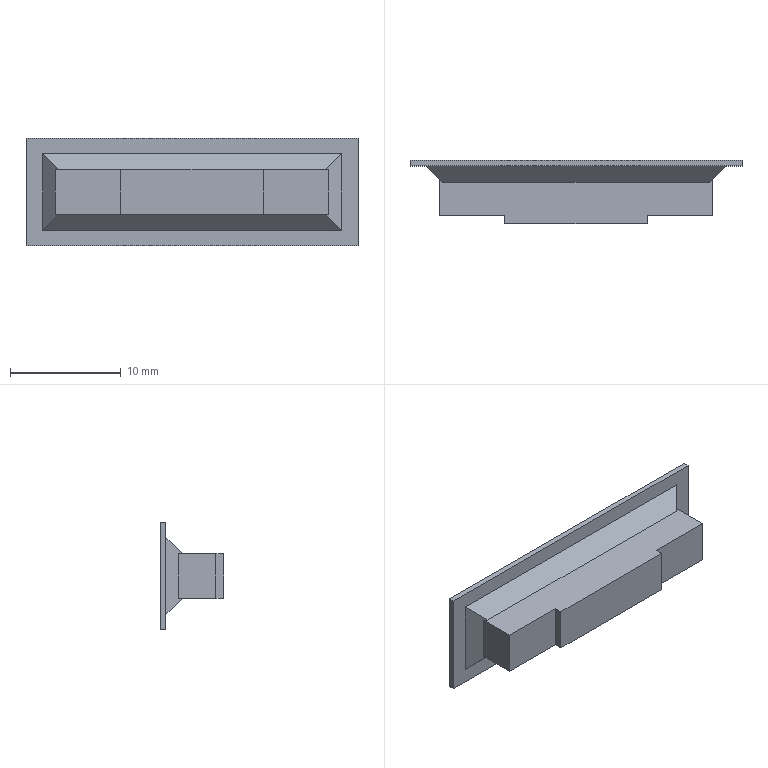Part | NX | 1 solid | 24 faces | box 30 x 5.7 x 9.7 mm | volume 631.13 mm3 | plane 24
STEP:
#1=CARTESIAN_POINT('',(12.05,-1.95,2.));
#2=VERTEX_POINT('',#1);
#3=CARTESIAN_POINT('',(-12.05,-1.95,2.));
#4=VERTEX_POINT('',#3);
#5=CARTESIAN_POINT('',(13.5,-1.95,2.));
#6=DIRECTION('',(-1.,0.,0.));
#7=VECTOR('',#6,1000.);
#8=LINE('',#5,#7);
#9=EDGE_CURVE('',#2,#4,#8,.T.);
#10=ORIENTED_EDGE('',*,*,#9,.F.);
#11=CARTESIAN_POINT('',(13.5,-0.5,3.45));
#12=VERTEX_POINT('',#11);
#13=CARTESIAN_POINT('',(13.5,-0.5,3.45));
#14=DIRECTION('',(0.5774,0.5774,0.5774));
#15=VECTOR('',#14,1000.);
#16=LINE('',#13,#15);
#17=EDGE_CURVE('',#2,#12,#16,.T.);
#18=ORIENTED_EDGE('',*,*,#17,.T.);
#19=CARTESIAN_POINT('',(-13.5,-0.5,3.45));
#20=VERTEX_POINT('',#19);
#21=CARTESIAN_POINT('',(13.5,-0.5,3.45));
#22=DIRECTION('',(-1.,0.,0.));
#23=VECTOR('',#22,1000.);
#24=LINE('',#21,#23);
#25=EDGE_CURVE('',#12,#20,#24,.T.);
#26=ORIENTED_EDGE('',*,*,#25,.T.);
#27=CARTESIAN_POINT('',(-4.5,-9.5,-5.55));
#28=DIRECTION('',(0.5774,-0.5774,-0.5774));
#29=VECTOR('',#28,1000.);
#30=LINE('',#27,#29);
#31=EDGE_CURVE('',#20,#4,#30,.T.);
#32=ORIENTED_EDGE('',*,*,#31,.T.);
#33=EDGE_LOOP('',(#10,#18,#26,#32));
#34=FACE_BOUND('',#33,.T.);
#35=CARTESIAN_POINT('',(13.5,-0.5,3.45));
#36=DIRECTION('',(0.,0.7071,-0.7071));
#37=DIRECTION('',(0.,0.7071,0.7071));
#38=AXIS2_PLACEMENT_3D('',#35,#36,#37);
#39=PLANE('',#38);
#40=ADVANCED_FACE('',(#34),#39,.F.);
#41=CARTESIAN_POINT('',(-12.05,-1.95,-2.));
#42=VERTEX_POINT('',#41);
#43=CARTESIAN_POINT('',(12.05,-1.95,-2.));
#44=VERTEX_POINT('',#43);
#45=CARTESIAN_POINT('',(13.5,-1.95,-2.));
#46=DIRECTION('',(1.,0.,0.));
#47=VECTOR('',#46,1000.);
#48=LINE('',#45,#47);
#49=EDGE_CURVE('',#42,#44,#48,.T.);
#50=ORIENTED_EDGE('',*,*,#49,.F.);
#51=CARTESIAN_POINT('',(-13.5,-0.5,-3.45));
#52=VERTEX_POINT('',#51);
#53=CARTESIAN_POINT('',(-4.5,-9.5,5.55));
#54=DIRECTION('',(-0.5774,0.5774,-0.5774));
#55=VECTOR('',#54,1000.);
#56=LINE('',#53,#55);
#57=EDGE_CURVE('',#42,#52,#56,.T.);
#58=ORIENTED_EDGE('',*,*,#57,.T.);
#59=CARTESIAN_POINT('',(13.5,-0.5,-3.45));
#60=VERTEX_POINT('',#59);
#61=CARTESIAN_POINT('',(13.5,-0.5,-3.45));
#62=DIRECTION('',(-1.,0.,0.));
#63=VECTOR('',#62,1000.);
#64=LINE('',#61,#63);
#65=EDGE_CURVE('',#60,#52,#64,.T.);
#66=ORIENTED_EDGE('',*,*,#65,.F.);
#67=CARTESIAN_POINT('',(13.5,-0.5,-3.45));
#68=DIRECTION('',(-0.5774,-0.5774,0.5774));
#69=VECTOR('',#68,1000.);
#70=LINE('',#67,#69);
#71=EDGE_CURVE('',#60,#44,#70,.T.);
#72=ORIENTED_EDGE('',*,*,#71,.T.);
#73=EDGE_LOOP('',(#50,#58,#66,#72));
#74=FACE_BOUND('',#73,.T.);
#75=CARTESIAN_POINT('',(13.5,-0.5,-3.45));
#76=DIRECTION('',(0.,0.7071,0.7071));
#77=DIRECTION('',(0.,-0.7071,0.7071));
#78=AXIS2_PLACEMENT_3D('',#75,#76,#77);
#79=PLANE('',#78);
#80=ADVANCED_FACE('',(#74),#79,.F.);
#81=CARTESIAN_POINT('',(12.35,-1.65,2.));
#82=VERTEX_POINT('',#81);
#83=CARTESIAN_POINT('',(13.5,-0.5,2.));
#84=DIRECTION('',(-0.7071,-0.7071,0.));
#85=VECTOR('',#84,1000.);
#86=LINE('',#83,#85);
#87=EDGE_CURVE('',#82,#2,#86,.T.);
#88=ORIENTED_EDGE('',*,*,#87,.F.);
#89=CARTESIAN_POINT('',(12.35,-1.65,-2.));
#90=VERTEX_POINT('',#89);
#91=CARTESIAN_POINT('',(12.35,-1.65,-4.85));
#92=DIRECTION('',(0.,0.,1.));
#93=VECTOR('',#92,1000.);
#94=LINE('',#91,#93);
#95=EDGE_CURVE('',#90,#82,#94,.T.);
#96=ORIENTED_EDGE('',*,*,#95,.F.);
#97=CARTESIAN_POINT('',(13.5,-0.5,-2.));
#98=DIRECTION('',(0.7071,0.7071,0.));
#99=VECTOR('',#98,1000.);
#100=LINE('',#97,#99);
#101=EDGE_CURVE('',#44,#90,#100,.T.);
#102=ORIENTED_EDGE('',*,*,#101,.F.);
#103=ORIENTED_EDGE('',*,*,#71,.F.);
#104=CARTESIAN_POINT('',(13.5,-0.5,3.45));
#105=DIRECTION('',(0.,0.,1.));
#106=VECTOR('',#105,1000.);
#107=LINE('',#104,#106);
#108=EDGE_CURVE('',#60,#12,#107,.T.);
#109=ORIENTED_EDGE('',*,*,#108,.T.);
#110=ORIENTED_EDGE('',*,*,#17,.F.);
#111=EDGE_LOOP('',(#88,#96,#102,#103,#109,#110));
#112=FACE_BOUND('',#111,.T.);
#113=CARTESIAN_POINT('',(13.5,-0.5,-4.85));
#114=DIRECTION('',(-0.7071,0.7071,0.));
#115=DIRECTION('',(-0.7071,-0.7071,0.));
#116=AXIS2_PLACEMENT_3D('',#113,#114,#115);
#117=PLANE('',#116);
#118=ADVANCED_FACE('',(#112),#117,.F.);
#119=CARTESIAN_POINT('',(-12.35,-1.65,2.));
#120=VERTEX_POINT('',#119);
#121=CARTESIAN_POINT('',(-13.5,-0.5,2.));
#122=DIRECTION('',(-0.7071,0.7071,0.));
#123=VECTOR('',#122,1000.);
#124=LINE('',#121,#123);
#125=EDGE_CURVE('',#4,#120,#124,.T.);
#126=ORIENTED_EDGE('',*,*,#125,.F.);
#127=ORIENTED_EDGE('',*,*,#31,.F.);
#128=CARTESIAN_POINT('',(-13.5,-0.5,3.45));
#129=DIRECTION('',(0.,0.,1.));
#130=VECTOR('',#129,1000.);
#131=LINE('',#128,#130);
#132=EDGE_CURVE('',#52,#20,#131,.T.);
#133=ORIENTED_EDGE('',*,*,#132,.F.);
#134=ORIENTED_EDGE('',*,*,#57,.F.);
#135=CARTESIAN_POINT('',(-12.35,-1.65,-2.));
#136=VERTEX_POINT('',#135);
#137=CARTESIAN_POINT('',(-13.5,-0.5,-2.));
#138=DIRECTION('',(0.7071,-0.7071,0.));
#139=VECTOR('',#138,1000.);
#140=LINE('',#137,#139);
#141=EDGE_CURVE('',#136,#42,#140,.T.);
#142=ORIENTED_EDGE('',*,*,#141,.F.);
#143=CARTESIAN_POINT('',(-12.35,-1.65,-4.85));
#144=DIRECTION('',(0.,0.,-1.));
#145=VECTOR('',#144,1000.);
#146=LINE('',#143,#145);
#147=EDGE_CURVE('',#120,#136,#146,.T.);
#148=ORIENTED_EDGE('',*,*,#147,.F.);
#149=EDGE_LOOP('',(#126,#127,#133,#134,#142,#148));
#150=FACE_BOUND('',#149,.T.);
#151=CARTESIAN_POINT('',(-13.5,-0.5,-4.85));
#152=DIRECTION('',(0.7071,0.7071,0.));
#153=DIRECTION('',(-0.7071,0.7071,0.));
#154=AXIS2_PLACEMENT_3D('',#151,#152,#153);
#155=PLANE('',#154);
#156=ADVANCED_FACE('',(#150),#155,.F.);
#157=ORIENTED_EDGE('',*,*,#132,.T.);
#158=ORIENTED_EDGE('',*,*,#25,.F.);
#159=ORIENTED_EDGE('',*,*,#108,.F.);
#160=ORIENTED_EDGE('',*,*,#65,.T.);
#161=EDGE_LOOP('',(#157,#158,#159,#160));
#162=FACE_BOUND('',#161,.T.);
#163=CARTESIAN_POINT('',(15.,-0.5,4.85));
#164=VERTEX_POINT('',#163);
#165=CARTESIAN_POINT('',(15.,-0.5,-4.85));
#166=VERTEX_POINT('',#165);
#167=CARTESIAN_POINT('',(15.,-0.5,-4.85));
#168=DIRECTION('',(0.,0.,-1.));
#169=VECTOR('',#168,1000.);
#170=LINE('',#167,#169);
#171=EDGE_CURVE('',#164,#166,#170,.T.);
#172=ORIENTED_EDGE('',*,*,#171,.F.);
#173=CARTESIAN_POINT('',(-15.,-0.5,4.85));
#174=VERTEX_POINT('',#173);
#175=CARTESIAN_POINT('',(-15.,-0.5,4.85));
#176=DIRECTION('',(1.,0.,0.));
#177=VECTOR('',#176,1000.);
#178=LINE('',#175,#177);
#179=EDGE_CURVE('',#174,#164,#178,.T.);
#180=ORIENTED_EDGE('',*,*,#179,.F.);
#181=CARTESIAN_POINT('',(-15.,-0.5,-4.85));
#182=VERTEX_POINT('',#181);
#183=CARTESIAN_POINT('',(-15.,-0.5,-4.85));
#184=DIRECTION('',(0.,0.,1.));
#185=VECTOR('',#184,1000.);
#186=LINE('',#183,#185);
#187=EDGE_CURVE('',#182,#174,#186,.T.);
#188=ORIENTED_EDGE('',*,*,#187,.F.);
#189=CARTESIAN_POINT('',(-15.,-0.5,-4.85));
#190=DIRECTION('',(-1.,0.,0.));
#191=VECTOR('',#190,1000.);
#192=LINE('',#189,#191);
#193=EDGE_CURVE('',#166,#182,#192,.T.);
#194=ORIENTED_EDGE('',*,*,#193,.F.);
#195=EDGE_LOOP('',(#172,#180,#188,#194));
#196=FACE_BOUND('',#195,.T.);
#197=CARTESIAN_POINT('',(-15.,-0.5,4.85));
#198=DIRECTION('',(0.,1.,0.));
#199=DIRECTION('',(0.,0.,1.));
#200=AXIS2_PLACEMENT_3D('',#197,#198,#199);
#201=PLANE('',#200);
#202=ADVANCED_FACE('',(#162,#196),#201,.F.);
#203=CARTESIAN_POINT('',(-15.,0.,-4.85));
#204=VERTEX_POINT('',#203);
#205=CARTESIAN_POINT('',(-15.,0.,4.85));
#206=VERTEX_POINT('',#205);
#207=CARTESIAN_POINT('',(-15.,0.,-4.85));
#208=DIRECTION('',(0.,0.,1.));
#209=VECTOR('',#208,1000.);
#210=LINE('',#207,#209);
#211=EDGE_CURVE('',#204,#206,#210,.T.);
#212=ORIENTED_EDGE('',*,*,#211,.F.);
#213=CARTESIAN_POINT('',(-15.,-0.5,-4.85));
#214=DIRECTION('',(0.,1.,0.));
#215=VECTOR('',#214,1000.);
#216=LINE('',#213,#215);
#217=EDGE_CURVE('',#182,#204,#216,.T.);
#218=ORIENTED_EDGE('',*,*,#217,.F.);
#219=ORIENTED_EDGE('',*,*,#187,.T.);
#220=CARTESIAN_POINT('',(-15.,-0.5,4.85));
#221=DIRECTION('',(0.,1.,0.));
#222=VECTOR('',#221,1000.);
#223=LINE('',#220,#222);
#224=EDGE_CURVE('',#174,#206,#223,.T.);
#225=ORIENTED_EDGE('',*,*,#224,.T.);
#226=EDGE_LOOP('',(#212,#218,#219,#225));
#227=FACE_BOUND('',#226,.T.);
#228=CARTESIAN_POINT('',(-15.,-0.5,-4.85));
#229=DIRECTION('',(-1.,0.,0.));
#230=DIRECTION('',(0.,0.,1.));
#231=AXIS2_PLACEMENT_3D('',#228,#229,#230);
#232=PLANE('',#231);
#233=ADVANCED_FACE('',(#227),#232,.T.);
#234=CARTESIAN_POINT('',(15.,0.,-4.85));
#235=VERTEX_POINT('',#234);
#236=CARTESIAN_POINT('',(-15.,0.,-4.85));
#237=DIRECTION('',(-1.,0.,0.));
#238=VECTOR('',#237,1000.);
#239=LINE('',#236,#238);
#240=EDGE_CURVE('',#235,#204,#239,.T.);
#241=ORIENTED_EDGE('',*,*,#240,.F.);
#242=CARTESIAN_POINT('',(15.,-0.5,-4.85));
#243=DIRECTION('',(0.,1.,0.));
#244=VECTOR('',#243,1000.);
#245=LINE('',#242,#244);
#246=EDGE_CURVE('',#166,#235,#245,.T.);
#247=ORIENTED_EDGE('',*,*,#246,.F.);
#248=ORIENTED_EDGE('',*,*,#193,.T.);
#249=ORIENTED_EDGE('',*,*,#217,.T.);
#250=EDGE_LOOP('',(#241,#247,#248,#249));
#251=FACE_BOUND('',#250,.T.);
#252=CARTESIAN_POINT('',(-15.,-0.5,-4.85));
#253=DIRECTION('',(0.,0.,-1.));
#254=DIRECTION('',(-1.,0.,0.));
#255=AXIS2_PLACEMENT_3D('',#252,#253,#254);
#256=PLANE('',#255);
#257=ADVANCED_FACE('',(#251),#256,.T.);
#258=CARTESIAN_POINT('',(15.,0.,4.85));
#259=VERTEX_POINT('',#258);
#260=CARTESIAN_POINT('',(15.,0.,-4.85));
#261=DIRECTION('',(0.,0.,-1.));
#262=VECTOR('',#261,1000.);
#263=LINE('',#260,#262);
#264=EDGE_CURVE('',#259,#235,#263,.T.);
#265=ORIENTED_EDGE('',*,*,#264,.F.);
#266=CARTESIAN_POINT('',(15.,-0.5,4.85));
#267=DIRECTION('',(0.,1.,0.));
#268=VECTOR('',#267,1000.);
#269=LINE('',#266,#268);
#270=EDGE_CURVE('',#164,#259,#269,.T.);
#271=ORIENTED_EDGE('',*,*,#270,.F.);
#272=ORIENTED_EDGE('',*,*,#171,.T.);
#273=ORIENTED_EDGE('',*,*,#246,.T.);
#274=EDGE_LOOP('',(#265,#271,#272,#273));
#275=FACE_BOUND('',#274,.T.);
#276=CARTESIAN_POINT('',(15.,-0.5,-4.85));
#277=DIRECTION('',(1.,0.,0.));
#278=DIRECTION('',(0.,0.,-1.));
#279=AXIS2_PLACEMENT_3D('',#276,#277,#278);
#280=PLANE('',#279);
#281=ADVANCED_FACE('',(#275),#280,.T.);
#282=CARTESIAN_POINT('',(-15.,0.,4.85));
#283=DIRECTION('',(1.,0.,0.));
#284=VECTOR('',#283,1000.);
#285=LINE('',#282,#284);
#286=EDGE_CURVE('',#206,#259,#285,.T.);
#287=ORIENTED_EDGE('',*,*,#286,.F.);
#288=ORIENTED_EDGE('',*,*,#224,.F.);
#289=ORIENTED_EDGE('',*,*,#179,.T.);
#290=ORIENTED_EDGE('',*,*,#270,.T.);
#291=EDGE_LOOP('',(#287,#288,#289,#290));
#292=FACE_BOUND('',#291,.T.);
#293=CARTESIAN_POINT('',(-15.,-0.5,4.85));
#294=DIRECTION('',(0.,0.,1.));
#295=DIRECTION('',(1.,0.,0.));
#296=AXIS2_PLACEMENT_3D('',#293,#294,#295);
#297=PLANE('',#296);
#298=ADVANCED_FACE('',(#292),#297,.T.);
#299=CARTESIAN_POINT('',(10.5,0.,2.1));
#300=VERTEX_POINT('',#299);
#301=CARTESIAN_POINT('',(10.5,0.,-2.1));
#302=VERTEX_POINT('',#301);
#303=CARTESIAN_POINT('',(10.5,0.,-2.1));
#304=DIRECTION('',(0.,0.,-1.));
#305=VECTOR('',#304,1000.);
#306=LINE('',#303,#305);
#307=EDGE_CURVE('',#300,#302,#306,.T.);
#308=ORIENTED_EDGE('',*,*,#307,.F.);
#309=CARTESIAN_POINT('',(-10.5,0.,2.1));
#310=VERTEX_POINT('',#309);
#311=CARTESIAN_POINT('',(10.5,0.,2.1));
#312=DIRECTION('',(1.,0.,0.));
#313=VECTOR('',#312,1000.);
#314=LINE('',#311,#313);
#315=EDGE_CURVE('',#310,#300,#314,.T.);
#316=ORIENTED_EDGE('',*,*,#315,.F.);
#317=CARTESIAN_POINT('',(-10.5,0.,-2.1));
#318=VERTEX_POINT('',#317);
#319=CARTESIAN_POINT('',(-10.5,0.,-2.1));
#320=DIRECTION('',(0.,0.,1.));
#321=VECTOR('',#320,1000.);
#322=LINE('',#319,#321);
#323=EDGE_CURVE('',#318,#310,#322,.T.);
#324=ORIENTED_EDGE('',*,*,#323,.F.);
#325=CARTESIAN_POINT('',(10.5,0.,-2.1));
#326=DIRECTION('',(-1.,0.,0.));
#327=VECTOR('',#326,1000.);
#328=LINE('',#325,#327);
#329=EDGE_CURVE('',#302,#318,#328,.T.);
#330=ORIENTED_EDGE('',*,*,#329,.F.);
#331=EDGE_LOOP('',(#308,#316,#324,#330));
#332=FACE_BOUND('',#331,.T.);
#333=ORIENTED_EDGE('',*,*,#211,.T.);
#334=ORIENTED_EDGE('',*,*,#286,.T.);
#335=ORIENTED_EDGE('',*,*,#264,.T.);
#336=ORIENTED_EDGE('',*,*,#240,.T.);
#337=EDGE_LOOP('',(#333,#334,#335,#336));
#338=FACE_BOUND('',#337,.T.);
#339=CARTESIAN_POINT('',(-15.,0.,4.85));
#340=DIRECTION('',(0.,1.,0.));
#341=DIRECTION('',(0.,0.,1.));
#342=AXIS2_PLACEMENT_3D('',#339,#340,#341);
#343=PLANE('',#342);
#344=ADVANCED_FACE('',(#332,#338),#343,.T.);
#345=CARTESIAN_POINT('',(12.35,-5.,2.));
#346=VERTEX_POINT('',#345);
#347=CARTESIAN_POINT('',(12.35,-5.7,2.));
#348=DIRECTION('',(0.,1.,0.));
#349=VECTOR('',#348,1000.);
#350=LINE('',#347,#349);
#351=EDGE_CURVE('',#346,#82,#350,.T.);
#352=ORIENTED_EDGE('',*,*,#351,.F.);
#353=CARTESIAN_POINT('',(12.35,-5.,-2.));
#354=VERTEX_POINT('',#353);
#355=CARTESIAN_POINT('',(12.35,-5.,-7.941));
#356=DIRECTION('',(0.,0.,1.));
#357=VECTOR('',#356,1000.);
#358=LINE('',#355,#357);
#359=EDGE_CURVE('',#354,#346,#358,.T.);
#360=ORIENTED_EDGE('',*,*,#359,.F.);
#361=CARTESIAN_POINT('',(12.35,-5.7,-2.));
#362=DIRECTION('',(0.,1.,0.));
#363=VECTOR('',#362,1000.);
#364=LINE('',#361,#363);
#365=EDGE_CURVE('',#354,#90,#364,.T.);
#366=ORIENTED_EDGE('',*,*,#365,.T.);
#367=ORIENTED_EDGE('',*,*,#95,.T.);
#368=EDGE_LOOP('',(#352,#360,#366,#367));
#369=FACE_BOUND('',#368,.T.);
#370=CARTESIAN_POINT('',(12.35,-5.7,2.));
#371=DIRECTION('',(-1.,0.,0.));
#372=DIRECTION('',(0.,0.,1.));
#373=AXIS2_PLACEMENT_3D('',#370,#371,#372);
#374=PLANE('',#373);
#375=ADVANCED_FACE('',(#369),#374,.F.);
#376=CARTESIAN_POINT('',(6.45,-5.,2.));
#377=VERTEX_POINT('',#376);
#378=CARTESIAN_POINT('',(6.45,-5.7,2.));
#379=VERTEX_POINT('',#378);
#380=CARTESIAN_POINT('',(6.45,-5.,2.));
#381=DIRECTION('',(0.,-1.,0.));
#382=VECTOR('',#381,1000.);
#383=LINE('',#380,#382);
#384=EDGE_CURVE('',#377,#379,#383,.T.);
#385=ORIENTED_EDGE('',*,*,#384,.F.);
#386=CARTESIAN_POINT('',(12.35,-5.,2.));
#387=DIRECTION('',(-1.,0.,0.));
#388=VECTOR('',#387,1000.);
#389=LINE('',#386,#388);
#390=EDGE_CURVE('',#346,#377,#389,.T.);
#391=ORIENTED_EDGE('',*,*,#390,.F.);
#392=ORIENTED_EDGE('',*,*,#351,.T.);
#393=ORIENTED_EDGE('',*,*,#87,.T.);
#394=ORIENTED_EDGE('',*,*,#9,.T.);
#395=ORIENTED_EDGE('',*,*,#125,.T.);
#396=CARTESIAN_POINT('',(-12.35,-5.,2.));
#397=VERTEX_POINT('',#396);
#398=CARTESIAN_POINT('',(-12.35,-5.7,2.));
#399=DIRECTION('',(0.,1.,0.));
#400=VECTOR('',#399,1000.);
#401=LINE('',#398,#400);
#402=EDGE_CURVE('',#397,#120,#401,.T.);
#403=ORIENTED_EDGE('',*,*,#402,.F.);
#404=CARTESIAN_POINT('',(-6.45,-5.,2.));
#405=VERTEX_POINT('',#404);
#406=CARTESIAN_POINT('',(-12.35,-5.,2.));
#407=DIRECTION('',(-1.,0.,0.));
#408=VECTOR('',#407,1000.);
#409=LINE('',#406,#408);
#410=EDGE_CURVE('',#405,#397,#409,.T.);
#411=ORIENTED_EDGE('',*,*,#410,.F.);
#412=CARTESIAN_POINT('',(-6.45,-5.7,2.));
#413=VERTEX_POINT('',#412);
#414=CARTESIAN_POINT('',(-6.45,-5.,2.));
#415=DIRECTION('',(0.,1.,0.));
#416=VECTOR('',#415,1000.);
#417=LINE('',#414,#416);
#418=EDGE_CURVE('',#413,#405,#417,.T.);
#419=ORIENTED_EDGE('',*,*,#418,.F.);
#420=CARTESIAN_POINT('',(12.35,-5.7,2.));
#421=DIRECTION('',(-1.,0.,0.));
#422=VECTOR('',#421,1000.);
#423=LINE('',#420,#422);
#424=EDGE_CURVE('',#379,#413,#423,.T.);
#425=ORIENTED_EDGE('',*,*,#424,.F.);
#426=EDGE_LOOP('',(#385,#391,#392,#393,#394,#395,#403,#411,#419,#425));
#427=FACE_BOUND('',#426,.T.);
#428=CARTESIAN_POINT('',(12.35,-5.7,2.));
#429=DIRECTION('',(0.,0.,-1.));
#430=DIRECTION('',(-1.,0.,0.));
#431=AXIS2_PLACEMENT_3D('',#428,#429,#430);
#432=PLANE('',#431);
#433=ADVANCED_FACE('',(#427),#432,.F.);
#434=CARTESIAN_POINT('',(-12.35,-5.,-2.));
#435=VERTEX_POINT('',#434);
#436=CARTESIAN_POINT('',(-12.35,-5.7,-2.));
#437=DIRECTION('',(0.,1.,0.));
#438=VECTOR('',#437,1000.);
#439=LINE('',#436,#438);
#440=EDGE_CURVE('',#435,#136,#439,.T.);
#441=ORIENTED_EDGE('',*,*,#440,.F.);
#442=CARTESIAN_POINT('',(-12.35,-5.,-7.941));
#443=DIRECTION('',(0.,0.,1.));
#444=VECTOR('',#443,1000.);
#445=LINE('',#442,#444);
#446=EDGE_CURVE('',#435,#397,#445,.T.);
#447=ORIENTED_EDGE('',*,*,#446,.T.);
#448=ORIENTED_EDGE('',*,*,#402,.T.);
#449=ORIENTED_EDGE('',*,*,#147,.T.);
#450=EDGE_LOOP('',(#441,#447,#448,#449));
#451=FACE_BOUND('',#450,.T.);
#452=CARTESIAN_POINT('',(-12.35,-5.7,2.));
#453=DIRECTION('',(1.,0.,0.));
#454=DIRECTION('',(0.,0.,-1.));
#455=AXIS2_PLACEMENT_3D('',#452,#453,#454);
#456=PLANE('',#455);
#457=ADVANCED_FACE('',(#451),#456,.F.);
#458=ORIENTED_EDGE('',*,*,#365,.F.);
#459=CARTESIAN_POINT('',(6.45,-5.,-2.));
#460=VERTEX_POINT('',#459);
#461=CARTESIAN_POINT('',(12.35,-5.,-2.));
#462=DIRECTION('',(1.,0.,0.));
#463=VECTOR('',#462,1000.);
#464=LINE('',#461,#463);
#465=EDGE_CURVE('',#460,#354,#464,.T.);
#466=ORIENTED_EDGE('',*,*,#465,.F.);
#467=CARTESIAN_POINT('',(6.45,-5.7,-2.));
#468=VERTEX_POINT('',#467);
#469=CARTESIAN_POINT('',(6.45,-5.,-2.));
#470=DIRECTION('',(0.,1.,0.));
#471=VECTOR('',#470,1000.);
#472=LINE('',#469,#471);
#473=EDGE_CURVE('',#468,#460,#472,.T.);
#474=ORIENTED_EDGE('',*,*,#473,.F.);
#475=CARTESIAN_POINT('',(-6.45,-5.7,-2.));
#476=VERTEX_POINT('',#475);
#477=CARTESIAN_POINT('',(12.35,-5.7,-2.));
#478=DIRECTION('',(1.,0.,0.));
#479=VECTOR('',#478,1000.);
#480=LINE('',#477,#479);
#481=EDGE_CURVE('',#476,#468,#480,.T.);
#482=ORIENTED_EDGE('',*,*,#481,.F.);
#483=CARTESIAN_POINT('',(-6.45,-5.,-2.));
#484=VERTEX_POINT('',#483);
#485=CARTESIAN_POINT('',(-6.45,-5.,-2.));
#486=DIRECTION('',(0.,-1.,0.));
#487=VECTOR('',#486,1000.);
#488=LINE('',#485,#487);
#489=EDGE_CURVE('',#484,#476,#488,.T.);
#490=ORIENTED_EDGE('',*,*,#489,.F.);
#491=CARTESIAN_POINT('',(-12.35,-5.,-2.));
#492=DIRECTION('',(1.,0.,0.));
#493=VECTOR('',#492,1000.);
#494=LINE('',#491,#493);
#495=EDGE_CURVE('',#435,#484,#494,.T.);
#496=ORIENTED_EDGE('',*,*,#495,.F.);
#497=ORIENTED_EDGE('',*,*,#440,.T.);
#498=ORIENTED_EDGE('',*,*,#141,.T.);
#499=ORIENTED_EDGE('',*,*,#49,.T.);
#500=ORIENTED_EDGE('',*,*,#101,.T.);
#501=EDGE_LOOP('',(#458,#466,#474,#482,#490,#496,#497,#498,#499,#500));
#502=FACE_BOUND('',#501,.T.);
#503=CARTESIAN_POINT('',(12.35,-5.7,-2.));
#504=DIRECTION('',(0.,0.,1.));
#505=DIRECTION('',(1.,0.,0.));
#506=AXIS2_PLACEMENT_3D('',#503,#504,#505);
#507=PLANE('',#506);
#508=ADVANCED_FACE('',(#502),#507,.F.);
#509=ORIENTED_EDGE('',*,*,#481,.T.);
#510=CARTESIAN_POINT('',(6.45,-5.7,-7.941));
#511=DIRECTION('',(0.,0.,1.));
#512=VECTOR('',#511,1000.);
#513=LINE('',#510,#512);
#514=EDGE_CURVE('',#468,#379,#513,.T.);
#515=ORIENTED_EDGE('',*,*,#514,.T.);
#516=ORIENTED_EDGE('',*,*,#424,.T.);
#517=CARTESIAN_POINT('',(-6.45,-5.7,-7.941));
#518=DIRECTION('',(0.,0.,1.));
#519=VECTOR('',#518,1000.);
#520=LINE('',#517,#519);
#521=EDGE_CURVE('',#476,#413,#520,.T.);
#522=ORIENTED_EDGE('',*,*,#521,.F.);
#523=EDGE_LOOP('',(#509,#515,#516,#522));
#524=FACE_BOUND('',#523,.T.);
#525=CARTESIAN_POINT('',(12.35,-5.7,-2.));
#526=DIRECTION('',(0.,1.,0.));
#527=DIRECTION('',(0.,0.,1.));
#528=AXIS2_PLACEMENT_3D('',#525,#526,#527);
#529=PLANE('',#528);
#530=ADVANCED_FACE('',(#524),#529,.F.);
#531=ORIENTED_EDGE('',*,*,#307,.T.);
#532=CARTESIAN_POINT('',(9.7,-0.8,-1.3));
#533=VERTEX_POINT('',#532);
#534=CARTESIAN_POINT('',(10.5,0.,-2.1));
#535=DIRECTION('',(0.5774,0.5774,-0.5774));
#536=VECTOR('',#535,1000.);
#537=LINE('',#534,#536);
#538=EDGE_CURVE('',#533,#302,#537,.T.);
#539=ORIENTED_EDGE('',*,*,#538,.F.);
#540=CARTESIAN_POINT('',(9.7,-0.8,1.3));
#541=VERTEX_POINT('',#540);
#542=CARTESIAN_POINT('',(9.7,-0.8,-2.1));
#543=DIRECTION('',(0.,0.,-1.));
#544=VECTOR('',#543,1000.);
#545=LINE('',#542,#544);
#546=EDGE_CURVE('',#541,#533,#545,.T.);
#547=ORIENTED_EDGE('',*,*,#546,.F.);
#548=CARTESIAN_POINT('',(10.5,0.,2.1));
#549=DIRECTION('',(0.5774,0.5774,0.5774));
#550=VECTOR('',#549,1000.);
#551=LINE('',#548,#550);
#552=EDGE_CURVE('',#541,#300,#551,.T.);
#553=ORIENTED_EDGE('',*,*,#552,.T.);
#554=EDGE_LOOP('',(#531,#539,#547,#553));
#555=FACE_BOUND('',#554,.T.);
#556=CARTESIAN_POINT('',(10.5,0.,-2.1));
#557=DIRECTION('',(0.7071,-0.7071,0.));
#558=DIRECTION('',(0.7071,0.7071,0.));
#559=AXIS2_PLACEMENT_3D('',#556,#557,#558);
#560=PLANE('',#559);
#561=ADVANCED_FACE('',(#555),#560,.F.);
#562=ORIENTED_EDGE('',*,*,#315,.T.);
#563=ORIENTED_EDGE('',*,*,#552,.F.);
#564=CARTESIAN_POINT('',(-9.7,-0.8,1.3));
#565=VERTEX_POINT('',#564);
#566=CARTESIAN_POINT('',(10.5,-0.8,1.3));
#567=DIRECTION('',(1.,0.,0.));
#568=VECTOR('',#567,1000.);
#569=LINE('',#566,#568);
#570=EDGE_CURVE('',#565,#541,#569,.T.);
#571=ORIENTED_EDGE('',*,*,#570,.F.);
#572=CARTESIAN_POINT('',(-9.1,-1.4,0.7));
#573=DIRECTION('',(-0.5774,0.5774,0.5774));
#574=VECTOR('',#573,1000.);
#575=LINE('',#572,#574);
#576=EDGE_CURVE('',#565,#310,#575,.T.);
#577=ORIENTED_EDGE('',*,*,#576,.T.);
#578=EDGE_LOOP('',(#562,#563,#571,#577));
#579=FACE_BOUND('',#578,.T.);
#580=CARTESIAN_POINT('',(10.5,0.,2.1));
#581=DIRECTION('',(0.,-0.7071,0.7071));
#582=DIRECTION('',(0.,-0.7071,-0.7071));
#583=AXIS2_PLACEMENT_3D('',#580,#581,#582);
#584=PLANE('',#583);
#585=ADVANCED_FACE('',(#579),#584,.F.);
#586=ORIENTED_EDGE('',*,*,#323,.T.);
#587=ORIENTED_EDGE('',*,*,#576,.F.);
#588=CARTESIAN_POINT('',(-9.7,-0.8,-1.3));
#589=VERTEX_POINT('',#588);
#590=CARTESIAN_POINT('',(-9.7,-0.8,-2.1));
#591=DIRECTION('',(0.,0.,1.));
#592=VECTOR('',#591,1000.);
#593=LINE('',#590,#592);
#594=EDGE_CURVE('',#589,#565,#593,.T.);
#595=ORIENTED_EDGE('',*,*,#594,.F.);
#596=CARTESIAN_POINT('',(-3.5,-7.,4.9));
#597=DIRECTION('',(-0.5774,0.5774,-0.5774));
#598=VECTOR('',#597,1000.);
#599=LINE('',#596,#598);
#600=EDGE_CURVE('',#589,#318,#599,.T.);
#601=ORIENTED_EDGE('',*,*,#600,.T.);
#602=EDGE_LOOP('',(#586,#587,#595,#601));
#603=FACE_BOUND('',#602,.T.);
#604=CARTESIAN_POINT('',(-10.5,0.,-2.1));
#605=DIRECTION('',(-0.7071,-0.7071,0.));
#606=DIRECTION('',(0.7071,-0.7071,0.));
#607=AXIS2_PLACEMENT_3D('',#604,#605,#606);
#608=PLANE('',#607);
#609=ADVANCED_FACE('',(#603),#608,.F.);
#610=ORIENTED_EDGE('',*,*,#329,.T.);
#611=ORIENTED_EDGE('',*,*,#600,.F.);
#612=CARTESIAN_POINT('',(10.5,-0.8,-1.3));
#613=DIRECTION('',(-1.,0.,0.));
#614=VECTOR('',#613,1000.);
#615=LINE('',#612,#614);
#616=EDGE_CURVE('',#533,#589,#615,.T.);
#617=ORIENTED_EDGE('',*,*,#616,.F.);
#618=ORIENTED_EDGE('',*,*,#538,.T.);
#619=EDGE_LOOP('',(#610,#611,#617,#618));
#620=FACE_BOUND('',#619,.T.);
#621=CARTESIAN_POINT('',(10.5,0.,-2.1));
#622=DIRECTION('',(0.,-0.7071,-0.7071));
#623=DIRECTION('',(0.,0.7071,-0.7071));
#624=AXIS2_PLACEMENT_3D('',#621,#622,#623);
#625=PLANE('',#624);
#626=ADVANCED_FACE('',(#620),#625,.F.);
#627=ORIENTED_EDGE('',*,*,#546,.T.);
#628=ORIENTED_EDGE('',*,*,#616,.T.);
#629=ORIENTED_EDGE('',*,*,#594,.T.);
#630=ORIENTED_EDGE('',*,*,#570,.T.);
#631=EDGE_LOOP('',(#627,#628,#629,#630));
#632=FACE_BOUND('',#631,.T.);
#633=CARTESIAN_POINT('',(10.5,-0.8,-2.1));
#634=DIRECTION('',(0.,-1.,0.));
#635=DIRECTION('',(0.,0.,-1.));
#636=AXIS2_PLACEMENT_3D('',#633,#634,#635);
#637=PLANE('',#636);
#638=ADVANCED_FACE('',(#632),#637,.F.);
#639=ORIENTED_EDGE('',*,*,#495,.T.);
#640=CARTESIAN_POINT('',(-6.45,-5.,-7.941));
#641=DIRECTION('',(0.,0.,1.));
#642=VECTOR('',#641,1000.);
#643=LINE('',#640,#642);
#644=EDGE_CURVE('',#484,#405,#643,.T.);
#645=ORIENTED_EDGE('',*,*,#644,.T.);
#646=ORIENTED_EDGE('',*,*,#410,.T.);
#647=ORIENTED_EDGE('',*,*,#446,.F.);
#648=EDGE_LOOP('',(#639,#645,#646,#647));
#649=FACE_BOUND('',#648,.T.);
#650=CARTESIAN_POINT('',(-12.35,-5.,-7.941));
#651=DIRECTION('',(0.,1.,0.));
#652=DIRECTION('',(0.,0.,1.));
#653=AXIS2_PLACEMENT_3D('',#650,#651,#652);
#654=PLANE('',#653);
#655=ADVANCED_FACE('',(#649),#654,.F.);
#656=ORIENTED_EDGE('',*,*,#489,.T.);
#657=ORIENTED_EDGE('',*,*,#521,.T.);
#658=ORIENTED_EDGE('',*,*,#418,.T.);
#659=ORIENTED_EDGE('',*,*,#644,.F.);
#660=EDGE_LOOP('',(#656,#657,#658,#659));
#661=FACE_BOUND('',#660,.T.);
#662=CARTESIAN_POINT('',(-6.45,-5.,-7.941));
#663=DIRECTION('',(1.,0.,0.));
#664=DIRECTION('',(0.,1.,0.));
#665=AXIS2_PLACEMENT_3D('',#662,#663,#664);
#666=PLANE('',#665);
#667=ADVANCED_FACE('',(#661),#666,.F.);
#668=ORIENTED_EDGE('',*,*,#465,.T.);
#669=ORIENTED_EDGE('',*,*,#359,.T.);
#670=ORIENTED_EDGE('',*,*,#390,.T.);
#671=CARTESIAN_POINT('',(6.45,-5.,-7.941));
#672=DIRECTION('',(0.,0.,1.));
#673=VECTOR('',#672,1000.);
#674=LINE('',#671,#673);
#675=EDGE_CURVE('',#460,#377,#674,.T.);
#676=ORIENTED_EDGE('',*,*,#675,.F.);
#677=EDGE_LOOP('',(#668,#669,#670,#676));
#678=FACE_BOUND('',#677,.T.);
#679=CARTESIAN_POINT('',(12.35,-5.,-7.941));
#680=DIRECTION('',(0.,1.,0.));
#681=DIRECTION('',(0.,0.,1.));
#682=AXIS2_PLACEMENT_3D('',#679,#680,#681);
#683=PLANE('',#682);
#684=ADVANCED_FACE('',(#678),#683,.F.);
#685=ORIENTED_EDGE('',*,*,#473,.T.);
#686=ORIENTED_EDGE('',*,*,#675,.T.);
#687=ORIENTED_EDGE('',*,*,#384,.T.);
#688=ORIENTED_EDGE('',*,*,#514,.F.);
#689=EDGE_LOOP('',(#685,#686,#687,#688));
#690=FACE_BOUND('',#689,.T.);
#691=CARTESIAN_POINT('',(6.45,-5.,-7.941));
#692=DIRECTION('',(-1.,0.,0.));
#693=DIRECTION('',(0.,-1.,0.));
#694=AXIS2_PLACEMENT_3D('',#691,#692,#693);
#695=PLANE('',#694);
#696=ADVANCED_FACE('',(#690),#695,.F.);
#697=CLOSED_SHELL('',(#40,#80,#118,#156,#202,#233,#257,#281,#298,#344,#375,#433,#457,#508,#530,#561,#585,#609,#626,#638,#655,#667,#684,#696));
#698=MANIFOLD_SOLID_BREP('',#697);
#699=(LENGTH_UNIT()NAMED_UNIT(*)SI_UNIT(.MILLI.,.METRE.));
#700=UNCERTAINTY_MEASURE_WITH_UNIT(LENGTH_MEASURE(0.00001),#699,'','');
#701=(NAMED_UNIT(*)PLANE_ANGLE_UNIT()SI_UNIT($,.RADIAN.));
#702=(NAMED_UNIT(*)SI_UNIT($,.STERADIAN.)SOLID_ANGLE_UNIT());
#703=(GEOMETRIC_REPRESENTATION_CONTEXT(3)GLOBAL_UNCERTAINTY_ASSIGNED_CONTEXT((#700))GLOBAL_UNIT_ASSIGNED_CONTEXT((#699,#701,#702))REPRESENTATION_CONTEXT('',''));
#704=ADVANCED_BREP_SHAPE_REPRESENTATION('',(#698),#703);